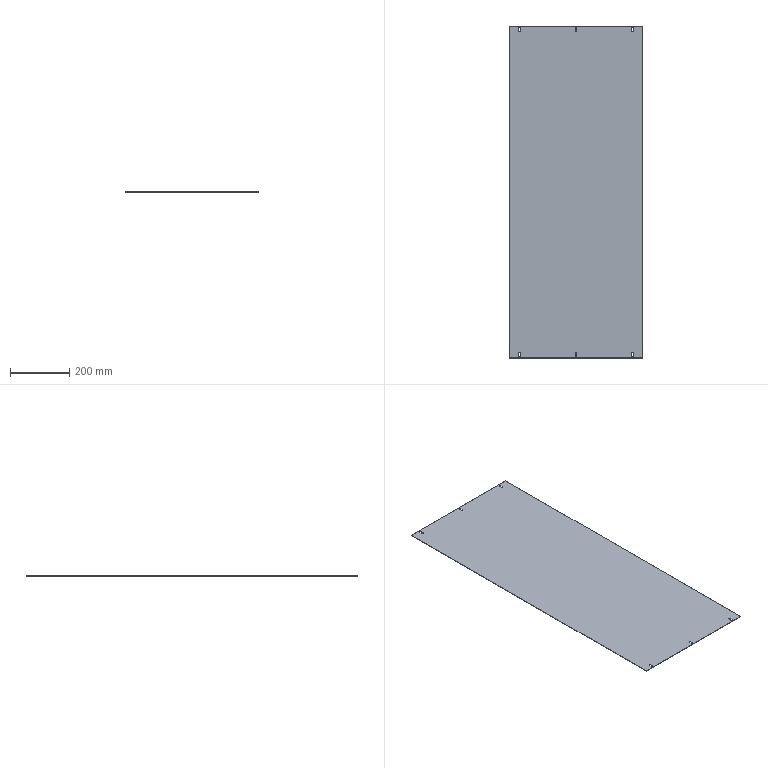Part | NX | features BREP 1 | 1 solid | 30 faces | box 450 x 1120 x 1.5 mm | volume 755314 mm3 | plane 18 | cylinder 12 | commonest cylinder face diameters 6 x12
STEP:
#1=CARTESIAN_POINT('',(-187.,544.,0.));
#2=VERTEX_POINT('',#1);
#3=CARTESIAN_POINT('',(-187.,544.,-1.5));
#4=VERTEX_POINT('',#3);
#5=CARTESIAN_POINT('',(-187.,544.,-14.));
#6=DIRECTION('',(0.,0.,-1.));
#7=VECTOR('',#6,1000.);
#8=LINE('',#5,#7);
#9=EDGE_CURVE('',#2,#4,#8,.T.);
#10=ORIENTED_EDGE('',*,*,#9,.F.);
#11=CARTESIAN_POINT('',(-187.,552.,0.));
#12=VERTEX_POINT('',#11);
#13=CARTESIAN_POINT('',(-187.,544.,0.));
#14=DIRECTION('',(0.,1.,0.));
#15=VECTOR('',#14,1000.);
#16=LINE('',#13,#15);
#17=EDGE_CURVE('',#2,#12,#16,.T.);
#18=ORIENTED_EDGE('',*,*,#17,.T.);
#19=CARTESIAN_POINT('',(-187.,552.,-1.5));
#20=VERTEX_POINT('',#19);
#21=CARTESIAN_POINT('',(-187.,552.,-14.));
#22=DIRECTION('',(0.,0.,-1.));
#23=VECTOR('',#22,1000.);
#24=LINE('',#21,#23);
#25=EDGE_CURVE('',#12,#20,#24,.T.);
#26=ORIENTED_EDGE('',*,*,#25,.T.);
#27=CARTESIAN_POINT('',(-187.,0.,-1.5));
#28=DIRECTION('',(0.,1.,0.));
#29=VECTOR('',#28,1000.);
#30=LINE('',#27,#29);
#31=EDGE_CURVE('',#4,#20,#30,.T.);
#32=ORIENTED_EDGE('',*,*,#31,.F.);
#33=EDGE_LOOP('',(#10,#18,#26,#32));
#34=FACE_BOUND('',#33,.T.);
#35=CARTESIAN_POINT('',(-187.,544.,-14.));
#36=DIRECTION('',(1.,0.,0.));
#37=DIRECTION('',(0.,0.,-1.));
#38=AXIS2_PLACEMENT_3D('',#35,#36,#37);
#39=PLANE('',#38);
#40=ADVANCED_FACE('',(#34),#39,.F.);
#41=CARTESIAN_POINT('',(-193.,552.,-1.5));
#42=VERTEX_POINT('',#41);
#43=CARTESIAN_POINT('',(-193.,552.,0.));
#44=VERTEX_POINT('',#43);
#45=CARTESIAN_POINT('',(-193.,552.,0.));
#46=DIRECTION('',(0.,0.,1.));
#47=VECTOR('',#46,1000.);
#48=LINE('',#45,#47);
#49=EDGE_CURVE('',#42,#44,#48,.T.);
#50=ORIENTED_EDGE('',*,*,#49,.T.);
#51=CARTESIAN_POINT('',(-193.,544.,0.));
#52=VERTEX_POINT('',#51);
#53=CARTESIAN_POINT('',(-193.,544.,0.));
#54=DIRECTION('',(0.,1.,0.));
#55=VECTOR('',#54,1000.);
#56=LINE('',#53,#55);
#57=EDGE_CURVE('',#52,#44,#56,.T.);
#58=ORIENTED_EDGE('',*,*,#57,.F.);
#59=CARTESIAN_POINT('',(-193.,544.,-1.5));
#60=VERTEX_POINT('',#59);
#61=CARTESIAN_POINT('',(-193.,544.,0.));
#62=DIRECTION('',(0.,0.,-1.));
#63=VECTOR('',#62,1000.);
#64=LINE('',#61,#63);
#65=EDGE_CURVE('',#52,#60,#64,.T.);
#66=ORIENTED_EDGE('',*,*,#65,.T.);
#67=CARTESIAN_POINT('',(-193.,0.,-1.5));
#68=DIRECTION('',(0.,-1.,0.));
#69=VECTOR('',#68,1000.);
#70=LINE('',#67,#69);
#71=EDGE_CURVE('',#42,#60,#70,.T.);
#72=ORIENTED_EDGE('',*,*,#71,.F.);
#73=EDGE_LOOP('',(#50,#58,#66,#72));
#74=FACE_BOUND('',#73,.T.);
#75=CARTESIAN_POINT('',(-193.,544.,0.));
#76=DIRECTION('',(-1.,0.,0.));
#77=DIRECTION('',(0.,0.,1.));
#78=AXIS2_PLACEMENT_3D('',#75,#76,#77);
#79=PLANE('',#78);
#80=ADVANCED_FACE('',(#74),#79,.F.);
#81=ORIENTED_EDGE('',*,*,#65,.F.);
#82=CARTESIAN_POINT('',(-190.,544.,0.));
#83=DIRECTION('',(0.,0.,1.));
#84=DIRECTION('',(1.,0.,0.));
#85=AXIS2_PLACEMENT_3D('',#82,#83,#84);
#86=CIRCLE('',#85,3.);
#87=EDGE_CURVE('',#52,#2,#86,.T.);
#88=ORIENTED_EDGE('',*,*,#87,.T.);
#89=ORIENTED_EDGE('',*,*,#9,.T.);
#90=CARTESIAN_POINT('',(-190.,544.,-1.5));
#91=DIRECTION('',(0.,0.,1.));
#92=DIRECTION('',(1.,0.,0.));
#93=AXIS2_PLACEMENT_3D('',#90,#91,#92);
#94=CIRCLE('',#93,3.);
#95=EDGE_CURVE('',#60,#4,#94,.T.);
#96=ORIENTED_EDGE('',*,*,#95,.F.);
#97=EDGE_LOOP('',(#81,#88,#89,#96));
#98=FACE_BOUND('',#97,.T.);
#99=CARTESIAN_POINT('',(-190.,544.,0.));
#100=DIRECTION('',(0.,0.,1.));
#101=DIRECTION('',(1.,0.,0.));
#102=AXIS2_PLACEMENT_3D('',#99,#100,#101);
#103=CYLINDRICAL_SURFACE('',#102,3.);
#104=ADVANCED_FACE('',(#98),#103,.F.);
#105=ORIENTED_EDGE('',*,*,#25,.F.);
#106=CARTESIAN_POINT('',(-190.,552.,0.));
#107=DIRECTION('',(0.,0.,1.));
#108=DIRECTION('',(1.,0.,0.));
#109=AXIS2_PLACEMENT_3D('',#106,#107,#108);
#110=CIRCLE('',#109,3.);
#111=EDGE_CURVE('',#12,#44,#110,.T.);
#112=ORIENTED_EDGE('',*,*,#111,.T.);
#113=ORIENTED_EDGE('',*,*,#49,.F.);
#114=CARTESIAN_POINT('',(-190.,552.,-1.5));
#115=DIRECTION('',(0.,0.,1.));
#116=DIRECTION('',(1.,0.,0.));
#117=AXIS2_PLACEMENT_3D('',#114,#115,#116);
#118=CIRCLE('',#117,3.);
#119=EDGE_CURVE('',#20,#42,#118,.T.);
#120=ORIENTED_EDGE('',*,*,#119,.F.);
#121=EDGE_LOOP('',(#105,#112,#113,#120));
#122=FACE_BOUND('',#121,.T.);
#123=CARTESIAN_POINT('',(-190.,552.,0.));
#124=DIRECTION('',(0.,0.,1.));
#125=DIRECTION('',(1.,0.,0.));
#126=AXIS2_PLACEMENT_3D('',#123,#124,#125);
#127=CYLINDRICAL_SURFACE('',#126,3.);
#128=ADVANCED_FACE('',(#122),#127,.F.);
#129=CARTESIAN_POINT('',(3.,544.,0.));
#130=VERTEX_POINT('',#129);
#131=CARTESIAN_POINT('',(3.,544.,-1.5));
#132=VERTEX_POINT('',#131);
#133=CARTESIAN_POINT('',(3.,544.,-14.));
#134=DIRECTION('',(0.,0.,-1.));
#135=VECTOR('',#134,1000.);
#136=LINE('',#133,#135);
#137=EDGE_CURVE('',#130,#132,#136,.T.);
#138=ORIENTED_EDGE('',*,*,#137,.F.);
#139=CARTESIAN_POINT('',(3.,552.,0.));
#140=VERTEX_POINT('',#139);
#141=CARTESIAN_POINT('',(3.,544.,0.));
#142=DIRECTION('',(0.,1.,0.));
#143=VECTOR('',#142,1000.);
#144=LINE('',#141,#143);
#145=EDGE_CURVE('',#130,#140,#144,.T.);
#146=ORIENTED_EDGE('',*,*,#145,.T.);
#147=CARTESIAN_POINT('',(3.,552.,-1.5));
#148=VERTEX_POINT('',#147);
#149=CARTESIAN_POINT('',(3.,552.,-14.));
#150=DIRECTION('',(0.,0.,-1.));
#151=VECTOR('',#150,1000.);
#152=LINE('',#149,#151);
#153=EDGE_CURVE('',#140,#148,#152,.T.);
#154=ORIENTED_EDGE('',*,*,#153,.T.);
#155=CARTESIAN_POINT('',(3.,0.,-1.5));
#156=DIRECTION('',(0.,1.,0.));
#157=VECTOR('',#156,1000.);
#158=LINE('',#155,#157);
#159=EDGE_CURVE('',#132,#148,#158,.T.);
#160=ORIENTED_EDGE('',*,*,#159,.F.);
#161=EDGE_LOOP('',(#138,#146,#154,#160));
#162=FACE_BOUND('',#161,.T.);
#163=CARTESIAN_POINT('',(3.,544.,-14.));
#164=DIRECTION('',(1.,0.,0.));
#165=DIRECTION('',(0.,0.,-1.));
#166=AXIS2_PLACEMENT_3D('',#163,#164,#165);
#167=PLANE('',#166);
#168=ADVANCED_FACE('',(#162),#167,.F.);
#169=CARTESIAN_POINT('',(-3.,544.,0.));
#170=VERTEX_POINT('',#169);
#171=CARTESIAN_POINT('',(-3.,544.,-1.5));
#172=VERTEX_POINT('',#171);
#173=CARTESIAN_POINT('',(-3.,544.,0.));
#174=DIRECTION('',(0.,0.,-1.));
#175=VECTOR('',#174,1000.);
#176=LINE('',#173,#175);
#177=EDGE_CURVE('',#170,#172,#176,.T.);
#178=ORIENTED_EDGE('',*,*,#177,.F.);
#179=CARTESIAN_POINT('',(0.,544.,0.));
#180=DIRECTION('',(0.,0.,1.));
#181=DIRECTION('',(1.,0.,0.));
#182=AXIS2_PLACEMENT_3D('',#179,#180,#181);
#183=CIRCLE('',#182,3.);
#184=EDGE_CURVE('',#170,#130,#183,.T.);
#185=ORIENTED_EDGE('',*,*,#184,.T.);
#186=ORIENTED_EDGE('',*,*,#137,.T.);
#187=CARTESIAN_POINT('',(0.,544.,-1.5));
#188=DIRECTION('',(0.,0.,1.));
#189=DIRECTION('',(1.,0.,0.));
#190=AXIS2_PLACEMENT_3D('',#187,#188,#189);
#191=CIRCLE('',#190,3.);
#192=EDGE_CURVE('',#172,#132,#191,.T.);
#193=ORIENTED_EDGE('',*,*,#192,.F.);
#194=EDGE_LOOP('',(#178,#185,#186,#193));
#195=FACE_BOUND('',#194,.T.);
#196=CARTESIAN_POINT('',(0.,544.,0.));
#197=DIRECTION('',(0.,0.,1.));
#198=DIRECTION('',(1.,0.,0.));
#199=AXIS2_PLACEMENT_3D('',#196,#197,#198);
#200=CYLINDRICAL_SURFACE('',#199,3.);
#201=ADVANCED_FACE('',(#195),#200,.F.);
#202=CARTESIAN_POINT('',(-3.,552.,-1.5));
#203=VERTEX_POINT('',#202);
#204=CARTESIAN_POINT('',(-3.,552.,0.));
#205=VERTEX_POINT('',#204);
#206=CARTESIAN_POINT('',(-3.,552.,0.));
#207=DIRECTION('',(0.,0.,1.));
#208=VECTOR('',#207,1000.);
#209=LINE('',#206,#208);
#210=EDGE_CURVE('',#203,#205,#209,.T.);
#211=ORIENTED_EDGE('',*,*,#210,.T.);
#212=CARTESIAN_POINT('',(-3.,544.,0.));
#213=DIRECTION('',(0.,1.,0.));
#214=VECTOR('',#213,1000.);
#215=LINE('',#212,#214);
#216=EDGE_CURVE('',#170,#205,#215,.T.);
#217=ORIENTED_EDGE('',*,*,#216,.F.);
#218=ORIENTED_EDGE('',*,*,#177,.T.);
#219=CARTESIAN_POINT('',(-3.,0.,-1.5));
#220=DIRECTION('',(0.,-1.,0.));
#221=VECTOR('',#220,1000.);
#222=LINE('',#219,#221);
#223=EDGE_CURVE('',#203,#172,#222,.T.);
#224=ORIENTED_EDGE('',*,*,#223,.F.);
#225=EDGE_LOOP('',(#211,#217,#218,#224));
#226=FACE_BOUND('',#225,.T.);
#227=CARTESIAN_POINT('',(-3.,544.,0.));
#228=DIRECTION('',(-1.,0.,0.));
#229=DIRECTION('',(0.,0.,1.));
#230=AXIS2_PLACEMENT_3D('',#227,#228,#229);
#231=PLANE('',#230);
#232=ADVANCED_FACE('',(#226),#231,.F.);
#233=ORIENTED_EDGE('',*,*,#153,.F.);
#234=CARTESIAN_POINT('',(0.,552.,0.));
#235=DIRECTION('',(0.,0.,1.));
#236=DIRECTION('',(1.,0.,0.));
#237=AXIS2_PLACEMENT_3D('',#234,#235,#236);
#238=CIRCLE('',#237,3.);
#239=EDGE_CURVE('',#140,#205,#238,.T.);
#240=ORIENTED_EDGE('',*,*,#239,.T.);
#241=ORIENTED_EDGE('',*,*,#210,.F.);
#242=CARTESIAN_POINT('',(0.,552.,-1.5));
#243=DIRECTION('',(0.,0.,1.));
#244=DIRECTION('',(1.,0.,0.));
#245=AXIS2_PLACEMENT_3D('',#242,#243,#244);
#246=CIRCLE('',#245,3.);
#247=EDGE_CURVE('',#148,#203,#246,.T.);
#248=ORIENTED_EDGE('',*,*,#247,.F.);
#249=EDGE_LOOP('',(#233,#240,#241,#248));
#250=FACE_BOUND('',#249,.T.);
#251=CARTESIAN_POINT('',(0.,552.,0.));
#252=DIRECTION('',(0.,0.,1.));
#253=DIRECTION('',(1.,0.,0.));
#254=AXIS2_PLACEMENT_3D('',#251,#252,#253);
#255=CYLINDRICAL_SURFACE('',#254,3.);
#256=ADVANCED_FACE('',(#250),#255,.F.);
#257=CARTESIAN_POINT('',(193.,544.,0.));
#258=VERTEX_POINT('',#257);
#259=CARTESIAN_POINT('',(193.,544.,-1.5));
#260=VERTEX_POINT('',#259);
#261=CARTESIAN_POINT('',(193.,544.,-14.));
#262=DIRECTION('',(0.,0.,-1.));
#263=VECTOR('',#262,1000.);
#264=LINE('',#261,#263);
#265=EDGE_CURVE('',#258,#260,#264,.T.);
#266=ORIENTED_EDGE('',*,*,#265,.F.);
#267=CARTESIAN_POINT('',(193.,552.,0.));
#268=VERTEX_POINT('',#267);
#269=CARTESIAN_POINT('',(193.,544.,0.));
#270=DIRECTION('',(0.,1.,0.));
#271=VECTOR('',#270,1000.);
#272=LINE('',#269,#271);
#273=EDGE_CURVE('',#258,#268,#272,.T.);
#274=ORIENTED_EDGE('',*,*,#273,.T.);
#275=CARTESIAN_POINT('',(193.,552.,-1.5));
#276=VERTEX_POINT('',#275);
#277=CARTESIAN_POINT('',(193.,552.,-14.));
#278=DIRECTION('',(0.,0.,-1.));
#279=VECTOR('',#278,1000.);
#280=LINE('',#277,#279);
#281=EDGE_CURVE('',#268,#276,#280,.T.);
#282=ORIENTED_EDGE('',*,*,#281,.T.);
#283=CARTESIAN_POINT('',(193.,0.,-1.5));
#284=DIRECTION('',(0.,1.,0.));
#285=VECTOR('',#284,1000.);
#286=LINE('',#283,#285);
#287=EDGE_CURVE('',#260,#276,#286,.T.);
#288=ORIENTED_EDGE('',*,*,#287,.F.);
#289=EDGE_LOOP('',(#266,#274,#282,#288));
#290=FACE_BOUND('',#289,.T.);
#291=CARTESIAN_POINT('',(193.,544.,-14.));
#292=DIRECTION('',(1.,0.,0.));
#293=DIRECTION('',(0.,0.,-1.));
#294=AXIS2_PLACEMENT_3D('',#291,#292,#293);
#295=PLANE('',#294);
#296=ADVANCED_FACE('',(#290),#295,.F.);
#297=CARTESIAN_POINT('',(187.,544.,0.));
#298=VERTEX_POINT('',#297);
#299=CARTESIAN_POINT('',(187.,544.,-1.5));
#300=VERTEX_POINT('',#299);
#301=CARTESIAN_POINT('',(187.,544.,0.));
#302=DIRECTION('',(0.,0.,-1.));
#303=VECTOR('',#302,1000.);
#304=LINE('',#301,#303);
#305=EDGE_CURVE('',#298,#300,#304,.T.);
#306=ORIENTED_EDGE('',*,*,#305,.F.);
#307=CARTESIAN_POINT('',(190.,544.,0.));
#308=DIRECTION('',(0.,0.,1.));
#309=DIRECTION('',(1.,0.,0.));
#310=AXIS2_PLACEMENT_3D('',#307,#308,#309);
#311=CIRCLE('',#310,3.);
#312=EDGE_CURVE('',#298,#258,#311,.T.);
#313=ORIENTED_EDGE('',*,*,#312,.T.);
#314=ORIENTED_EDGE('',*,*,#265,.T.);
#315=CARTESIAN_POINT('',(190.,544.,-1.5));
#316=DIRECTION('',(0.,0.,1.));
#317=DIRECTION('',(1.,0.,0.));
#318=AXIS2_PLACEMENT_3D('',#315,#316,#317);
#319=CIRCLE('',#318,3.);
#320=EDGE_CURVE('',#300,#260,#319,.T.);
#321=ORIENTED_EDGE('',*,*,#320,.F.);
#322=EDGE_LOOP('',(#306,#313,#314,#321));
#323=FACE_BOUND('',#322,.T.);
#324=CARTESIAN_POINT('',(190.,544.,0.));
#325=DIRECTION('',(0.,0.,1.));
#326=DIRECTION('',(1.,0.,0.));
#327=AXIS2_PLACEMENT_3D('',#324,#325,#326);
#328=CYLINDRICAL_SURFACE('',#327,3.);
#329=ADVANCED_FACE('',(#323),#328,.F.);
#330=CARTESIAN_POINT('',(187.,552.,-1.5));
#331=VERTEX_POINT('',#330);
#332=CARTESIAN_POINT('',(187.,552.,0.));
#333=VERTEX_POINT('',#332);
#334=CARTESIAN_POINT('',(187.,552.,0.));
#335=DIRECTION('',(0.,0.,1.));
#336=VECTOR('',#335,1000.);
#337=LINE('',#334,#336);
#338=EDGE_CURVE('',#331,#333,#337,.T.);
#339=ORIENTED_EDGE('',*,*,#338,.T.);
#340=CARTESIAN_POINT('',(187.,544.,0.));
#341=DIRECTION('',(0.,1.,0.));
#342=VECTOR('',#341,1000.);
#343=LINE('',#340,#342);
#344=EDGE_CURVE('',#298,#333,#343,.T.);
#345=ORIENTED_EDGE('',*,*,#344,.F.);
#346=ORIENTED_EDGE('',*,*,#305,.T.);
#347=CARTESIAN_POINT('',(187.,0.,-1.5));
#348=DIRECTION('',(0.,-1.,0.));
#349=VECTOR('',#348,1000.);
#350=LINE('',#347,#349);
#351=EDGE_CURVE('',#331,#300,#350,.T.);
#352=ORIENTED_EDGE('',*,*,#351,.F.);
#353=EDGE_LOOP('',(#339,#345,#346,#352));
#354=FACE_BOUND('',#353,.T.);
#355=CARTESIAN_POINT('',(187.,544.,0.));
#356=DIRECTION('',(-1.,0.,0.));
#357=DIRECTION('',(0.,0.,1.));
#358=AXIS2_PLACEMENT_3D('',#355,#356,#357);
#359=PLANE('',#358);
#360=ADVANCED_FACE('',(#354),#359,.F.);
#361=ORIENTED_EDGE('',*,*,#281,.F.);
#362=CARTESIAN_POINT('',(190.,552.,0.));
#363=DIRECTION('',(0.,0.,1.));
#364=DIRECTION('',(1.,0.,0.));
#365=AXIS2_PLACEMENT_3D('',#362,#363,#364);
#366=CIRCLE('',#365,3.);
#367=EDGE_CURVE('',#268,#333,#366,.T.);
#368=ORIENTED_EDGE('',*,*,#367,.T.);
#369=ORIENTED_EDGE('',*,*,#338,.F.);
#370=CARTESIAN_POINT('',(190.,552.,-1.5));
#371=DIRECTION('',(0.,0.,1.));
#372=DIRECTION('',(1.,0.,0.));
#373=AXIS2_PLACEMENT_3D('',#370,#371,#372);
#374=CIRCLE('',#373,3.);
#375=EDGE_CURVE('',#276,#331,#374,.T.);
#376=ORIENTED_EDGE('',*,*,#375,.F.);
#377=EDGE_LOOP('',(#361,#368,#369,#376));
#378=FACE_BOUND('',#377,.T.);
#379=CARTESIAN_POINT('',(190.,552.,0.));
#380=DIRECTION('',(0.,0.,1.));
#381=DIRECTION('',(1.,0.,0.));
#382=AXIS2_PLACEMENT_3D('',#379,#380,#381);
#383=CYLINDRICAL_SURFACE('',#382,3.);
#384=ADVANCED_FACE('',(#378),#383,.F.);
#385=CARTESIAN_POINT('',(-187.,-552.,0.));
#386=VERTEX_POINT('',#385);
#387=CARTESIAN_POINT('',(-187.,-552.,-1.5));
#388=VERTEX_POINT('',#387);
#389=CARTESIAN_POINT('',(-187.,-552.,-14.));
#390=DIRECTION('',(0.,0.,-1.));
#391=VECTOR('',#390,1000.);
#392=LINE('',#389,#391);
#393=EDGE_CURVE('',#386,#388,#392,.T.);
#394=ORIENTED_EDGE('',*,*,#393,.F.);
#395=CARTESIAN_POINT('',(-187.,-544.,0.));
#396=VERTEX_POINT('',#395);
#397=CARTESIAN_POINT('',(-187.,-552.,0.));
#398=DIRECTION('',(0.,1.,0.));
#399=VECTOR('',#398,1000.);
#400=LINE('',#397,#399);
#401=EDGE_CURVE('',#386,#396,#400,.T.);
#402=ORIENTED_EDGE('',*,*,#401,.T.);
#403=CARTESIAN_POINT('',(-187.,-544.,-1.5));
#404=VERTEX_POINT('',#403);
#405=CARTESIAN_POINT('',(-187.,-544.,-14.));
#406=DIRECTION('',(0.,0.,-1.));
#407=VECTOR('',#406,1000.);
#408=LINE('',#405,#407);
#409=EDGE_CURVE('',#396,#404,#408,.T.);
#410=ORIENTED_EDGE('',*,*,#409,.T.);
#411=CARTESIAN_POINT('',(-187.,0.,-1.5));
#412=DIRECTION('',(0.,1.,0.));
#413=VECTOR('',#412,1000.);
#414=LINE('',#411,#413);
#415=EDGE_CURVE('',#388,#404,#414,.T.);
#416=ORIENTED_EDGE('',*,*,#415,.F.);
#417=EDGE_LOOP('',(#394,#402,#410,#416));
#418=FACE_BOUND('',#417,.T.);
#419=CARTESIAN_POINT('',(-187.,-552.,-14.));
#420=DIRECTION('',(1.,0.,0.));
#421=DIRECTION('',(0.,0.,-1.));
#422=AXIS2_PLACEMENT_3D('',#419,#420,#421);
#423=PLANE('',#422);
#424=ADVANCED_FACE('',(#418),#423,.F.);
#425=CARTESIAN_POINT('',(-193.,-544.,-1.5));
#426=VERTEX_POINT('',#425);
#427=CARTESIAN_POINT('',(-193.,-544.,0.));
#428=VERTEX_POINT('',#427);
#429=CARTESIAN_POINT('',(-193.,-544.,0.));
#430=DIRECTION('',(0.,0.,1.));
#431=VECTOR('',#430,1000.);
#432=LINE('',#429,#431);
#433=EDGE_CURVE('',#426,#428,#432,.T.);
#434=ORIENTED_EDGE('',*,*,#433,.T.);
#435=CARTESIAN_POINT('',(-193.,-552.,0.));
#436=VERTEX_POINT('',#435);
#437=CARTESIAN_POINT('',(-193.,-552.,0.));
#438=DIRECTION('',(0.,1.,0.));
#439=VECTOR('',#438,1000.);
#440=LINE('',#437,#439);
#441=EDGE_CURVE('',#436,#428,#440,.T.);
#442=ORIENTED_EDGE('',*,*,#441,.F.);
#443=CARTESIAN_POINT('',(-193.,-552.,-1.5));
#444=VERTEX_POINT('',#443);
#445=CARTESIAN_POINT('',(-193.,-552.,0.));
#446=DIRECTION('',(0.,0.,-1.));
#447=VECTOR('',#446,1000.);
#448=LINE('',#445,#447);
#449=EDGE_CURVE('',#436,#444,#448,.T.);
#450=ORIENTED_EDGE('',*,*,#449,.T.);
#451=CARTESIAN_POINT('',(-193.,0.,-1.5));
#452=DIRECTION('',(0.,-1.,0.));
#453=VECTOR('',#452,1000.);
#454=LINE('',#451,#453);
#455=EDGE_CURVE('',#426,#444,#454,.T.);
#456=ORIENTED_EDGE('',*,*,#455,.F.);
#457=EDGE_LOOP('',(#434,#442,#450,#456));
#458=FACE_BOUND('',#457,.T.);
#459=CARTESIAN_POINT('',(-193.,-552.,0.));
#460=DIRECTION('',(-1.,0.,0.));
#461=DIRECTION('',(0.,0.,1.));
#462=AXIS2_PLACEMENT_3D('',#459,#460,#461);
#463=PLANE('',#462);
#464=ADVANCED_FACE('',(#458),#463,.F.);
#465=ORIENTED_EDGE('',*,*,#449,.F.);
#466=CARTESIAN_POINT('',(-190.,-552.,0.));
#467=DIRECTION('',(0.,0.,1.));
#468=DIRECTION('',(1.,0.,0.));
#469=AXIS2_PLACEMENT_3D('',#466,#467,#468);
#470=CIRCLE('',#469,3.);
#471=EDGE_CURVE('',#436,#386,#470,.T.);
#472=ORIENTED_EDGE('',*,*,#471,.T.);
#473=ORIENTED_EDGE('',*,*,#393,.T.);
#474=CARTESIAN_POINT('',(-190.,-552.,-1.5));
#475=DIRECTION('',(0.,0.,1.));
#476=DIRECTION('',(1.,0.,0.));
#477=AXIS2_PLACEMENT_3D('',#474,#475,#476);
#478=CIRCLE('',#477,3.);
#479=EDGE_CURVE('',#444,#388,#478,.T.);
#480=ORIENTED_EDGE('',*,*,#479,.F.);
#481=EDGE_LOOP('',(#465,#472,#473,#480));
#482=FACE_BOUND('',#481,.T.);
#483=CARTESIAN_POINT('',(-190.,-552.,0.));
#484=DIRECTION('',(0.,0.,1.));
#485=DIRECTION('',(1.,0.,0.));
#486=AXIS2_PLACEMENT_3D('',#483,#484,#485);
#487=CYLINDRICAL_SURFACE('',#486,3.);
#488=ADVANCED_FACE('',(#482),#487,.F.);
#489=ORIENTED_EDGE('',*,*,#409,.F.);
#490=CARTESIAN_POINT('',(-190.,-544.,0.));
#491=DIRECTION('',(0.,0.,1.));
#492=DIRECTION('',(1.,0.,0.));
#493=AXIS2_PLACEMENT_3D('',#490,#491,#492);
#494=CIRCLE('',#493,3.);
#495=EDGE_CURVE('',#396,#428,#494,.T.);
#496=ORIENTED_EDGE('',*,*,#495,.T.);
#497=ORIENTED_EDGE('',*,*,#433,.F.);
#498=CARTESIAN_POINT('',(-190.,-544.,-1.5));
#499=DIRECTION('',(0.,0.,1.));
#500=DIRECTION('',(1.,0.,0.));
#501=AXIS2_PLACEMENT_3D('',#498,#499,#500);
#502=CIRCLE('',#501,3.);
#503=EDGE_CURVE('',#404,#426,#502,.T.);
#504=ORIENTED_EDGE('',*,*,#503,.F.);
#505=EDGE_LOOP('',(#489,#496,#497,#504));
#506=FACE_BOUND('',#505,.T.);
#507=CARTESIAN_POINT('',(-190.,-544.,0.));
#508=DIRECTION('',(0.,0.,1.));
#509=DIRECTION('',(1.,0.,0.));
#510=AXIS2_PLACEMENT_3D('',#507,#508,#509);
#511=CYLINDRICAL_SURFACE('',#510,3.);
#512=ADVANCED_FACE('',(#506),#511,.F.);
#513=CARTESIAN_POINT('',(3.,-552.,0.));
#514=VERTEX_POINT('',#513);
#515=CARTESIAN_POINT('',(3.,-552.,-1.5));
#516=VERTEX_POINT('',#515);
#517=CARTESIAN_POINT('',(3.,-552.,-14.));
#518=DIRECTION('',(0.,0.,-1.));
#519=VECTOR('',#518,1000.);
#520=LINE('',#517,#519);
#521=EDGE_CURVE('',#514,#516,#520,.T.);
#522=ORIENTED_EDGE('',*,*,#521,.F.);
#523=CARTESIAN_POINT('',(3.,-544.,0.));
#524=VERTEX_POINT('',#523);
#525=CARTESIAN_POINT('',(3.,-552.,0.));
#526=DIRECTION('',(0.,1.,0.));
#527=VECTOR('',#526,1000.);
#528=LINE('',#525,#527);
#529=EDGE_CURVE('',#514,#524,#528,.T.);
#530=ORIENTED_EDGE('',*,*,#529,.T.);
#531=CARTESIAN_POINT('',(3.,-544.,-1.5));
#532=VERTEX_POINT('',#531);
#533=CARTESIAN_POINT('',(3.,-544.,-14.));
#534=DIRECTION('',(0.,0.,-1.));
#535=VECTOR('',#534,1000.);
#536=LINE('',#533,#535);
#537=EDGE_CURVE('',#524,#532,#536,.T.);
#538=ORIENTED_EDGE('',*,*,#537,.T.);
#539=CARTESIAN_POINT('',(3.,0.,-1.5));
#540=DIRECTION('',(0.,1.,0.));
#541=VECTOR('',#540,1000.);
#542=LINE('',#539,#541);
#543=EDGE_CURVE('',#516,#532,#542,.T.);
#544=ORIENTED_EDGE('',*,*,#543,.F.);
#545=EDGE_LOOP('',(#522,#530,#538,#544));
#546=FACE_BOUND('',#545,.T.);
#547=CARTESIAN_POINT('',(3.,-552.,-14.));
#548=DIRECTION('',(1.,0.,0.));
#549=DIRECTION('',(0.,0.,-1.));
#550=AXIS2_PLACEMENT_3D('',#547,#548,#549);
#551=PLANE('',#550);
#552=ADVANCED_FACE('',(#546),#551,.F.);
#553=CARTESIAN_POINT('',(-3.,-552.,0.));
#554=VERTEX_POINT('',#553);
#555=CARTESIAN_POINT('',(-3.,-552.,-1.5));
#556=VERTEX_POINT('',#555);
#557=CARTESIAN_POINT('',(-3.,-552.,0.));
#558=DIRECTION('',(0.,0.,-1.));
#559=VECTOR('',#558,1000.);
#560=LINE('',#557,#559);
#561=EDGE_CURVE('',#554,#556,#560,.T.);
#562=ORIENTED_EDGE('',*,*,#561,.F.);
#563=CARTESIAN_POINT('',(0.,-552.,0.));
#564=DIRECTION('',(0.,0.,1.));
#565=DIRECTION('',(1.,0.,0.));
#566=AXIS2_PLACEMENT_3D('',#563,#564,#565);
#567=CIRCLE('',#566,3.);
#568=EDGE_CURVE('',#554,#514,#567,.T.);
#569=ORIENTED_EDGE('',*,*,#568,.T.);
#570=ORIENTED_EDGE('',*,*,#521,.T.);
#571=CARTESIAN_POINT('',(0.,-552.,-1.5));
#572=DIRECTION('',(0.,0.,1.));
#573=DIRECTION('',(1.,0.,0.));
#574=AXIS2_PLACEMENT_3D('',#571,#572,#573);
#575=CIRCLE('',#574,3.);
#576=EDGE_CURVE('',#556,#516,#575,.T.);
#577=ORIENTED_EDGE('',*,*,#576,.F.);
#578=EDGE_LOOP('',(#562,#569,#570,#577));
#579=FACE_BOUND('',#578,.T.);
#580=CARTESIAN_POINT('',(0.,-552.,0.));
#581=DIRECTION('',(0.,0.,1.));
#582=DIRECTION('',(1.,0.,0.));
#583=AXIS2_PLACEMENT_3D('',#580,#581,#582);
#584=CYLINDRICAL_SURFACE('',#583,3.);
#585=ADVANCED_FACE('',(#579),#584,.F.);
#586=CARTESIAN_POINT('',(-3.,-544.,-1.5));
#587=VERTEX_POINT('',#586);
#588=CARTESIAN_POINT('',(-3.,-544.,0.));
#589=VERTEX_POINT('',#588);
#590=CARTESIAN_POINT('',(-3.,-544.,0.));
#591=DIRECTION('',(0.,0.,1.));
#592=VECTOR('',#591,1000.);
#593=LINE('',#590,#592);
#594=EDGE_CURVE('',#587,#589,#593,.T.);
#595=ORIENTED_EDGE('',*,*,#594,.T.);
#596=CARTESIAN_POINT('',(-3.,-552.,0.));
#597=DIRECTION('',(0.,1.,0.));
#598=VECTOR('',#597,1000.);
#599=LINE('',#596,#598);
#600=EDGE_CURVE('',#554,#589,#599,.T.);
#601=ORIENTED_EDGE('',*,*,#600,.F.);
#602=ORIENTED_EDGE('',*,*,#561,.T.);
#603=CARTESIAN_POINT('',(-3.,0.,-1.5));
#604=DIRECTION('',(0.,-1.,0.));
#605=VECTOR('',#604,1000.);
#606=LINE('',#603,#605);
#607=EDGE_CURVE('',#587,#556,#606,.T.);
#608=ORIENTED_EDGE('',*,*,#607,.F.);
#609=EDGE_LOOP('',(#595,#601,#602,#608));
#610=FACE_BOUND('',#609,.T.);
#611=CARTESIAN_POINT('',(-3.,-552.,0.));
#612=DIRECTION('',(-1.,0.,0.));
#613=DIRECTION('',(0.,0.,1.));
#614=AXIS2_PLACEMENT_3D('',#611,#612,#613);
#615=PLANE('',#614);
#616=ADVANCED_FACE('',(#610),#615,.F.);
#617=ORIENTED_EDGE('',*,*,#537,.F.);
#618=CARTESIAN_POINT('',(0.,-544.,0.));
#619=DIRECTION('',(0.,0.,1.));
#620=DIRECTION('',(1.,0.,0.));
#621=AXIS2_PLACEMENT_3D('',#618,#619,#620);
#622=CIRCLE('',#621,3.);
#623=EDGE_CURVE('',#524,#589,#622,.T.);
#624=ORIENTED_EDGE('',*,*,#623,.T.);
#625=ORIENTED_EDGE('',*,*,#594,.F.);
#626=CARTESIAN_POINT('',(0.,-544.,-1.5));
#627=DIRECTION('',(0.,0.,1.));
#628=DIRECTION('',(1.,0.,0.));
#629=AXIS2_PLACEMENT_3D('',#626,#627,#628);
#630=CIRCLE('',#629,3.);
#631=EDGE_CURVE('',#532,#587,#630,.T.);
#632=ORIENTED_EDGE('',*,*,#631,.F.);
#633=EDGE_LOOP('',(#617,#624,#625,#632));
#634=FACE_BOUND('',#633,.T.);
#635=CARTESIAN_POINT('',(0.,-544.,0.));
#636=DIRECTION('',(0.,0.,1.));
#637=DIRECTION('',(1.,0.,0.));
#638=AXIS2_PLACEMENT_3D('',#635,#636,#637);
#639=CYLINDRICAL_SURFACE('',#638,3.);
#640=ADVANCED_FACE('',(#634),#639,.F.);
#641=CARTESIAN_POINT('',(193.,-552.,0.));
#642=VERTEX_POINT('',#641);
#643=CARTESIAN_POINT('',(193.,-552.,-1.5));
#644=VERTEX_POINT('',#643);
#645=CARTESIAN_POINT('',(193.,-552.,-14.));
#646=DIRECTION('',(0.,0.,-1.));
#647=VECTOR('',#646,1000.);
#648=LINE('',#645,#647);
#649=EDGE_CURVE('',#642,#644,#648,.T.);
#650=ORIENTED_EDGE('',*,*,#649,.F.);
#651=CARTESIAN_POINT('',(193.,-544.,0.));
#652=VERTEX_POINT('',#651);
#653=CARTESIAN_POINT('',(193.,-552.,0.));
#654=DIRECTION('',(0.,1.,0.));
#655=VECTOR('',#654,1000.);
#656=LINE('',#653,#655);
#657=EDGE_CURVE('',#642,#652,#656,.T.);
#658=ORIENTED_EDGE('',*,*,#657,.T.);
#659=CARTESIAN_POINT('',(193.,-544.,-1.5));
#660=VERTEX_POINT('',#659);
#661=CARTESIAN_POINT('',(193.,-544.,-14.));
#662=DIRECTION('',(0.,0.,-1.));
#663=VECTOR('',#662,1000.);
#664=LINE('',#661,#663);
#665=EDGE_CURVE('',#652,#660,#664,.T.);
#666=ORIENTED_EDGE('',*,*,#665,.T.);
#667=CARTESIAN_POINT('',(193.,0.,-1.5));
#668=DIRECTION('',(0.,1.,0.));
#669=VECTOR('',#668,1000.);
#670=LINE('',#667,#669);
#671=EDGE_CURVE('',#644,#660,#670,.T.);
#672=ORIENTED_EDGE('',*,*,#671,.F.);
#673=EDGE_LOOP('',(#650,#658,#666,#672));
#674=FACE_BOUND('',#673,.T.);
#675=CARTESIAN_POINT('',(193.,-552.,-14.));
#676=DIRECTION('',(1.,0.,0.));
#677=DIRECTION('',(0.,0.,-1.));
#678=AXIS2_PLACEMENT_3D('',#675,#676,#677);
#679=PLANE('',#678);
#680=ADVANCED_FACE('',(#674),#679,.F.);
#681=CARTESIAN_POINT('',(187.,-544.,-1.5));
#682=VERTEX_POINT('',#681);
#683=CARTESIAN_POINT('',(187.,-544.,0.));
#684=VERTEX_POINT('',#683);
#685=CARTESIAN_POINT('',(187.,-544.,0.));
#686=DIRECTION('',(0.,0.,1.));
#687=VECTOR('',#686,1000.);
#688=LINE('',#685,#687);
#689=EDGE_CURVE('',#682,#684,#688,.T.);
#690=ORIENTED_EDGE('',*,*,#689,.T.);
#691=CARTESIAN_POINT('',(187.,-552.,0.));
#692=VERTEX_POINT('',#691);
#693=CARTESIAN_POINT('',(187.,-552.,0.));
#694=DIRECTION('',(0.,1.,0.));
#695=VECTOR('',#694,1000.);
#696=LINE('',#693,#695);
#697=EDGE_CURVE('',#692,#684,#696,.T.);
#698=ORIENTED_EDGE('',*,*,#697,.F.);
#699=CARTESIAN_POINT('',(187.,-552.,-1.5));
#700=VERTEX_POINT('',#699);
#701=CARTESIAN_POINT('',(187.,-552.,0.));
#702=DIRECTION('',(0.,0.,-1.));
#703=VECTOR('',#702,1000.);
#704=LINE('',#701,#703);
#705=EDGE_CURVE('',#692,#700,#704,.T.);
#706=ORIENTED_EDGE('',*,*,#705,.T.);
#707=CARTESIAN_POINT('',(187.,0.,-1.5));
#708=DIRECTION('',(0.,-1.,0.));
#709=VECTOR('',#708,1000.);
#710=LINE('',#707,#709);
#711=EDGE_CURVE('',#682,#700,#710,.T.);
#712=ORIENTED_EDGE('',*,*,#711,.F.);
#713=EDGE_LOOP('',(#690,#698,#706,#712));
#714=FACE_BOUND('',#713,.T.);
#715=CARTESIAN_POINT('',(187.,-552.,0.));
#716=DIRECTION('',(-1.,0.,0.));
#717=DIRECTION('',(0.,0.,1.));
#718=AXIS2_PLACEMENT_3D('',#715,#716,#717);
#719=PLANE('',#718);
#720=ADVANCED_FACE('',(#714),#719,.F.);
#721=ORIENTED_EDGE('',*,*,#705,.F.);
#722=CARTESIAN_POINT('',(190.,-552.,0.));
#723=DIRECTION('',(0.,0.,1.));
#724=DIRECTION('',(1.,0.,0.));
#725=AXIS2_PLACEMENT_3D('',#722,#723,#724);
#726=CIRCLE('',#725,3.);
#727=EDGE_CURVE('',#692,#642,#726,.T.);
#728=ORIENTED_EDGE('',*,*,#727,.T.);
#729=ORIENTED_EDGE('',*,*,#649,.T.);
#730=CARTESIAN_POINT('',(190.,-552.,-1.5));
#731=DIRECTION('',(0.,0.,1.));
#732=DIRECTION('',(1.,0.,0.));
#733=AXIS2_PLACEMENT_3D('',#730,#731,#732);
#734=CIRCLE('',#733,3.);
#735=EDGE_CURVE('',#700,#644,#734,.T.);
#736=ORIENTED_EDGE('',*,*,#735,.F.);
#737=EDGE_LOOP('',(#721,#728,#729,#736));
#738=FACE_BOUND('',#737,.T.);
#739=CARTESIAN_POINT('',(190.,-552.,0.));
#740=DIRECTION('',(0.,0.,1.));
#741=DIRECTION('',(1.,0.,0.));
#742=AXIS2_PLACEMENT_3D('',#739,#740,#741);
#743=CYLINDRICAL_SURFACE('',#742,3.);
#744=ADVANCED_FACE('',(#738),#743,.F.);
#745=ORIENTED_EDGE('',*,*,#665,.F.);
#746=CARTESIAN_POINT('',(190.,-544.,0.));
#747=DIRECTION('',(0.,0.,1.));
#748=DIRECTION('',(1.,0.,0.));
#749=AXIS2_PLACEMENT_3D('',#746,#747,#748);
#750=CIRCLE('',#749,3.);
#751=EDGE_CURVE('',#652,#684,#750,.T.);
#752=ORIENTED_EDGE('',*,*,#751,.T.);
#753=ORIENTED_EDGE('',*,*,#689,.F.);
#754=CARTESIAN_POINT('',(190.,-544.,-1.5));
#755=DIRECTION('',(0.,0.,1.));
#756=DIRECTION('',(1.,0.,0.));
#757=AXIS2_PLACEMENT_3D('',#754,#755,#756);
#758=CIRCLE('',#757,3.);
#759=EDGE_CURVE('',#660,#682,#758,.T.);
#760=ORIENTED_EDGE('',*,*,#759,.F.);
#761=EDGE_LOOP('',(#745,#752,#753,#760));
#762=FACE_BOUND('',#761,.T.);
#763=CARTESIAN_POINT('',(190.,-544.,0.));
#764=DIRECTION('',(0.,0.,1.));
#765=DIRECTION('',(1.,0.,0.));
#766=AXIS2_PLACEMENT_3D('',#763,#764,#765);
#767=CYLINDRICAL_SURFACE('',#766,3.);
#768=ADVANCED_FACE('',(#762),#767,.F.);
#769=CARTESIAN_POINT('',(-225.,560.,-1.5));
#770=VERTEX_POINT('',#769);
#771=CARTESIAN_POINT('',(-225.,-560.,-1.5));
#772=VERTEX_POINT('',#771);
#773=CARTESIAN_POINT('',(-225.,-560.,-1.5));
#774=DIRECTION('',(0.,-1.,0.));
#775=VECTOR('',#774,1000.);
#776=LINE('',#773,#775);
#777=EDGE_CURVE('',#770,#772,#776,.T.);
#778=ORIENTED_EDGE('',*,*,#777,.F.);
#779=CARTESIAN_POINT('',(225.,560.,-1.5));
#780=VERTEX_POINT('',#779);
#781=CARTESIAN_POINT('',(225.,560.,-1.5));
#782=DIRECTION('',(-1.,0.,0.));
#783=VECTOR('',#782,1000.);
#784=LINE('',#781,#783);
#785=EDGE_CURVE('',#780,#770,#784,.T.);
#786=ORIENTED_EDGE('',*,*,#785,.F.);
#787=CARTESIAN_POINT('',(225.,-560.,-1.5));
#788=VERTEX_POINT('',#787);
#789=CARTESIAN_POINT('',(225.,-560.,-1.5));
#790=DIRECTION('',(0.,1.,0.));
#791=VECTOR('',#790,1000.);
#792=LINE('',#789,#791);
#793=EDGE_CURVE('',#788,#780,#792,.T.);
#794=ORIENTED_EDGE('',*,*,#793,.F.);
#795=CARTESIAN_POINT('',(225.,-560.,-1.5));
#796=DIRECTION('',(1.,0.,0.));
#797=VECTOR('',#796,1000.);
#798=LINE('',#795,#797);
#799=EDGE_CURVE('',#772,#788,#798,.T.);
#800=ORIENTED_EDGE('',*,*,#799,.F.);
#801=EDGE_LOOP('',(#778,#786,#794,#800));
#802=FACE_BOUND('',#801,.T.);
#803=ORIENTED_EDGE('',*,*,#759,.T.);
#804=ORIENTED_EDGE('',*,*,#711,.T.);
#805=ORIENTED_EDGE('',*,*,#735,.T.);
#806=ORIENTED_EDGE('',*,*,#671,.T.);
#807=EDGE_LOOP('',(#803,#804,#805,#806));
#808=FACE_BOUND('',#807,.T.);
#809=ORIENTED_EDGE('',*,*,#543,.T.);
#810=ORIENTED_EDGE('',*,*,#631,.T.);
#811=ORIENTED_EDGE('',*,*,#607,.T.);
#812=ORIENTED_EDGE('',*,*,#576,.T.);
#813=EDGE_LOOP('',(#809,#810,#811,#812));
#814=FACE_BOUND('',#813,.T.);
#815=ORIENTED_EDGE('',*,*,#503,.T.);
#816=ORIENTED_EDGE('',*,*,#455,.T.);
#817=ORIENTED_EDGE('',*,*,#479,.T.);
#818=ORIENTED_EDGE('',*,*,#415,.T.);
#819=EDGE_LOOP('',(#815,#816,#817,#818));
#820=FACE_BOUND('',#819,.T.);
#821=ORIENTED_EDGE('',*,*,#287,.T.);
#822=ORIENTED_EDGE('',*,*,#375,.T.);
#823=ORIENTED_EDGE('',*,*,#351,.T.);
#824=ORIENTED_EDGE('',*,*,#320,.T.);
#825=EDGE_LOOP('',(#821,#822,#823,#824));
#826=FACE_BOUND('',#825,.T.);
#827=ORIENTED_EDGE('',*,*,#159,.T.);
#828=ORIENTED_EDGE('',*,*,#247,.T.);
#829=ORIENTED_EDGE('',*,*,#223,.T.);
#830=ORIENTED_EDGE('',*,*,#192,.T.);
#831=EDGE_LOOP('',(#827,#828,#829,#830));
#832=FACE_BOUND('',#831,.T.);
#833=ORIENTED_EDGE('',*,*,#119,.T.);
#834=ORIENTED_EDGE('',*,*,#71,.T.);
#835=ORIENTED_EDGE('',*,*,#95,.T.);
#836=ORIENTED_EDGE('',*,*,#31,.T.);
#837=EDGE_LOOP('',(#833,#834,#835,#836));
#838=FACE_BOUND('',#837,.T.);
#839=CARTESIAN_POINT('',(0.,0.,-1.5));
#840=DIRECTION('',(0.,0.,1.));
#841=DIRECTION('',(1.,0.,0.));
#842=AXIS2_PLACEMENT_3D('',#839,#840,#841);
#843=PLANE('',#842);
#844=ADVANCED_FACE('',(#802,#808,#814,#820,#826,#832,#838),#843,.F.);
#845=CARTESIAN_POINT('',(-225.,-560.,0.));
#846=VERTEX_POINT('',#845);
#847=CARTESIAN_POINT('',(225.,-560.,0.));
#848=VERTEX_POINT('',#847);
#849=CARTESIAN_POINT('',(225.,-560.,0.));
#850=DIRECTION('',(1.,0.,0.));
#851=VECTOR('',#850,1000.);
#852=LINE('',#849,#851);
#853=EDGE_CURVE('',#846,#848,#852,.T.);
#854=ORIENTED_EDGE('',*,*,#853,.F.);
#855=CARTESIAN_POINT('',(-225.,-560.,-1.5));
#856=DIRECTION('',(0.,0.,1.));
#857=VECTOR('',#856,1000.);
#858=LINE('',#855,#857);
#859=EDGE_CURVE('',#772,#846,#858,.T.);
#860=ORIENTED_EDGE('',*,*,#859,.F.);
#861=ORIENTED_EDGE('',*,*,#799,.T.);
#862=CARTESIAN_POINT('',(225.,-560.,-1.5));
#863=DIRECTION('',(0.,0.,1.));
#864=VECTOR('',#863,1000.);
#865=LINE('',#862,#864);
#866=EDGE_CURVE('',#788,#848,#865,.T.);
#867=ORIENTED_EDGE('',*,*,#866,.T.);
#868=EDGE_LOOP('',(#854,#860,#861,#867));
#869=FACE_BOUND('',#868,.T.);
#870=CARTESIAN_POINT('',(225.,-560.,-1.5));
#871=DIRECTION('',(0.,-1.,0.));
#872=DIRECTION('',(0.,0.,-1.));
#873=AXIS2_PLACEMENT_3D('',#870,#871,#872);
#874=PLANE('',#873);
#875=ADVANCED_FACE('',(#869),#874,.T.);
#876=CARTESIAN_POINT('',(225.,560.,0.));
#877=VERTEX_POINT('',#876);
#878=CARTESIAN_POINT('',(225.,-560.,0.));
#879=DIRECTION('',(0.,1.,0.));
#880=VECTOR('',#879,1000.);
#881=LINE('',#878,#880);
#882=EDGE_CURVE('',#848,#877,#881,.T.);
#883=ORIENTED_EDGE('',*,*,#882,.F.);
#884=ORIENTED_EDGE('',*,*,#866,.F.);
#885=ORIENTED_EDGE('',*,*,#793,.T.);
#886=CARTESIAN_POINT('',(225.,560.,-1.5));
#887=DIRECTION('',(0.,0.,1.));
#888=VECTOR('',#887,1000.);
#889=LINE('',#886,#888);
#890=EDGE_CURVE('',#780,#877,#889,.T.);
#891=ORIENTED_EDGE('',*,*,#890,.T.);
#892=EDGE_LOOP('',(#883,#884,#885,#891));
#893=FACE_BOUND('',#892,.T.);
#894=CARTESIAN_POINT('',(225.,-560.,-1.5));
#895=DIRECTION('',(1.,0.,0.));
#896=DIRECTION('',(0.,0.,-1.));
#897=AXIS2_PLACEMENT_3D('',#894,#895,#896);
#898=PLANE('',#897);
#899=ADVANCED_FACE('',(#893),#898,.T.);
#900=CARTESIAN_POINT('',(-225.,560.,0.));
#901=VERTEX_POINT('',#900);
#902=CARTESIAN_POINT('',(225.,560.,0.));
#903=DIRECTION('',(-1.,0.,0.));
#904=VECTOR('',#903,1000.);
#905=LINE('',#902,#904);
#906=EDGE_CURVE('',#877,#901,#905,.T.);
#907=ORIENTED_EDGE('',*,*,#906,.F.);
#908=ORIENTED_EDGE('',*,*,#890,.F.);
#909=ORIENTED_EDGE('',*,*,#785,.T.);
#910=CARTESIAN_POINT('',(-225.,560.,-1.5));
#911=DIRECTION('',(0.,0.,1.));
#912=VECTOR('',#911,1000.);
#913=LINE('',#910,#912);
#914=EDGE_CURVE('',#770,#901,#913,.T.);
#915=ORIENTED_EDGE('',*,*,#914,.T.);
#916=EDGE_LOOP('',(#907,#908,#909,#915));
#917=FACE_BOUND('',#916,.T.);
#918=CARTESIAN_POINT('',(225.,560.,-1.5));
#919=DIRECTION('',(0.,1.,0.));
#920=DIRECTION('',(-1.,0.,0.));
#921=AXIS2_PLACEMENT_3D('',#918,#919,#920);
#922=PLANE('',#921);
#923=ADVANCED_FACE('',(#917),#922,.T.);
#924=CARTESIAN_POINT('',(-225.,-560.,0.));
#925=DIRECTION('',(0.,-1.,0.));
#926=VECTOR('',#925,1000.);
#927=LINE('',#924,#926);
#928=EDGE_CURVE('',#901,#846,#927,.T.);
#929=ORIENTED_EDGE('',*,*,#928,.F.);
#930=ORIENTED_EDGE('',*,*,#914,.F.);
#931=ORIENTED_EDGE('',*,*,#777,.T.);
#932=ORIENTED_EDGE('',*,*,#859,.T.);
#933=EDGE_LOOP('',(#929,#930,#931,#932));
#934=FACE_BOUND('',#933,.T.);
#935=CARTESIAN_POINT('',(-225.,-560.,-1.5));
#936=DIRECTION('',(-1.,0.,0.));
#937=DIRECTION('',(0.,-1.,0.));
#938=AXIS2_PLACEMENT_3D('',#935,#936,#937);
#939=PLANE('',#938);
#940=ADVANCED_FACE('',(#934),#939,.T.);
#941=ORIENTED_EDGE('',*,*,#727,.F.);
#942=ORIENTED_EDGE('',*,*,#697,.T.);
#943=ORIENTED_EDGE('',*,*,#751,.F.);
#944=ORIENTED_EDGE('',*,*,#657,.F.);
#945=EDGE_LOOP('',(#941,#942,#943,#944));
#946=FACE_BOUND('',#945,.T.);
#947=ORIENTED_EDGE('',*,*,#928,.T.);
#948=ORIENTED_EDGE('',*,*,#853,.T.);
#949=ORIENTED_EDGE('',*,*,#882,.T.);
#950=ORIENTED_EDGE('',*,*,#906,.T.);
#951=EDGE_LOOP('',(#947,#948,#949,#950));
#952=FACE_BOUND('',#951,.T.);
#953=ORIENTED_EDGE('',*,*,#623,.F.);
#954=ORIENTED_EDGE('',*,*,#529,.F.);
#955=ORIENTED_EDGE('',*,*,#568,.F.);
#956=ORIENTED_EDGE('',*,*,#600,.T.);
#957=EDGE_LOOP('',(#953,#954,#955,#956));
#958=FACE_BOUND('',#957,.T.);
#959=ORIENTED_EDGE('',*,*,#495,.F.);
#960=ORIENTED_EDGE('',*,*,#401,.F.);
#961=ORIENTED_EDGE('',*,*,#471,.F.);
#962=ORIENTED_EDGE('',*,*,#441,.T.);
#963=EDGE_LOOP('',(#959,#960,#961,#962));
#964=FACE_BOUND('',#963,.T.);
#965=ORIENTED_EDGE('',*,*,#367,.F.);
#966=ORIENTED_EDGE('',*,*,#273,.F.);
#967=ORIENTED_EDGE('',*,*,#312,.F.);
#968=ORIENTED_EDGE('',*,*,#344,.T.);
#969=EDGE_LOOP('',(#965,#966,#967,#968));
#970=FACE_BOUND('',#969,.T.);
#971=ORIENTED_EDGE('',*,*,#239,.F.);
#972=ORIENTED_EDGE('',*,*,#145,.F.);
#973=ORIENTED_EDGE('',*,*,#184,.F.);
#974=ORIENTED_EDGE('',*,*,#216,.T.);
#975=EDGE_LOOP('',(#971,#972,#973,#974));
#976=FACE_BOUND('',#975,.T.);
#977=ORIENTED_EDGE('',*,*,#17,.F.);
#978=ORIENTED_EDGE('',*,*,#87,.F.);
#979=ORIENTED_EDGE('',*,*,#57,.T.);
#980=ORIENTED_EDGE('',*,*,#111,.F.);
#981=EDGE_LOOP('',(#977,#978,#979,#980));
#982=FACE_BOUND('',#981,.T.);
#983=CARTESIAN_POINT('',(0.,0.,0.));
#984=DIRECTION('',(0.,0.,1.));
#985=DIRECTION('',(1.,0.,0.));
#986=AXIS2_PLACEMENT_3D('',#983,#984,#985);
#987=PLANE('',#986);
#988=ADVANCED_FACE('',(#946,#952,#958,#964,#970,#976,#982),#987,.T.);
#989=CLOSED_SHELL('',(#40,#80,#104,#128,#168,#201,#232,#256,#296,#329,#360,#384,#424,#464,#488,#512,#552,#585,#616,#640,#680,#720,#744,#768,#844,#875,#899,#923,#940,#988));
#990=MANIFOLD_SOLID_BREP('',#989);
#991=(LENGTH_UNIT()NAMED_UNIT(*)SI_UNIT(.MILLI.,.METRE.));
#992=UNCERTAINTY_MEASURE_WITH_UNIT(LENGTH_MEASURE(0.00001),#991,'','');
#993=(NAMED_UNIT(*)PLANE_ANGLE_UNIT()SI_UNIT($,.RADIAN.));
#994=(NAMED_UNIT(*)SI_UNIT($,.STERADIAN.)SOLID_ANGLE_UNIT());
#995=(GEOMETRIC_REPRESENTATION_CONTEXT(3)GLOBAL_UNCERTAINTY_ASSIGNED_CONTEXT((#992))GLOBAL_UNIT_ASSIGNED_CONTEXT((#991,#993,#994))REPRESENTATION_CONTEXT('',''));
#996=ADVANCED_BREP_SHAPE_REPRESENTATION('',(#990),#995);